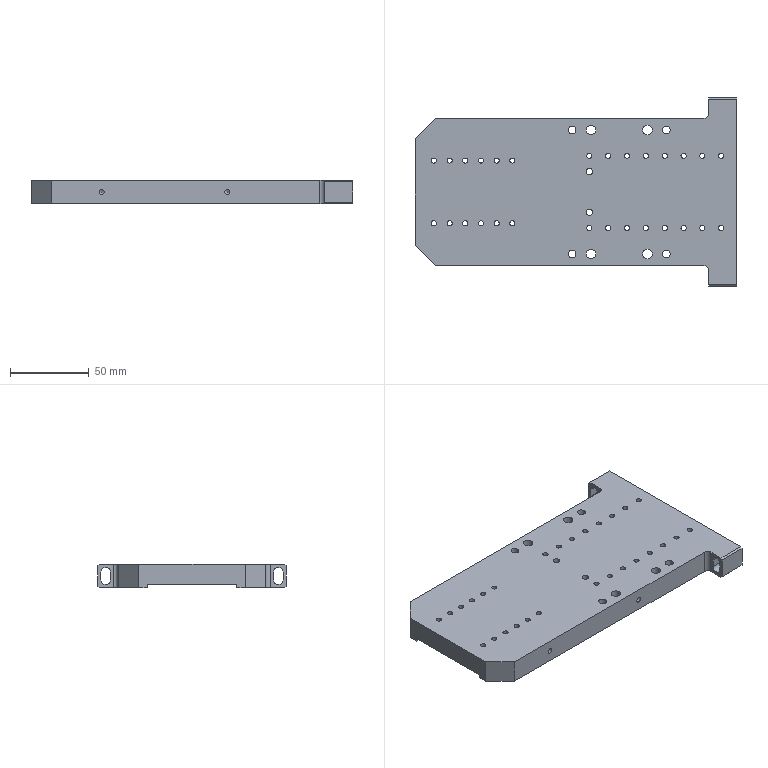CAM job | NX | 3-axis milling, drilling | part box 205 x 120 x 15 mm | stock box 210 x 120 x 20 mm
Tools:
number,name,description,diameter,corner_radius,flute_length,length,flutes
9,D10,平底铣刀-粗,10.0,0.0,35.0,75.0,2
7,D6-J,平底铣刀-精,6.0,0.0,25.0,75.0,2
10,D10-J,平底铣刀-精,10.0,0.0,35.0,75.0,2
1,D80R0.8FLYCUTTER,圆鼻刀-粗,80.0,0.8,50.0,75.0,2
1,D80R0.8FLYCUTTER-J,圆鼻刀-精,80.0,0.8,50.0,75.0,2
2,D6CHAMFERTOOL,倒角刀,6.0,0.0,3.0,25.0,2
21,M4X0.7,丝锥,3.3,0.0,35.0,50.0,2
23,M6X1.0,丝锥,5.0,0.0,35.0,50.0,2
19,D4REAMER,Drilling Tool,4.0,0.0,75.0,100.0,6
20,D6REAMER,Drilling Tool,6.0,0.0,75.0,100.0,6
15,ZT5,钻头,5.0,0.0,35.0,50.0,2
13,DRILL3.3,Twist Drill 3.3 mm,3.3,0.0,35.0,35.008,2
17,ZT3.9,Drilling Tool,3.9,0.0,35.0,50.0,2
18,ZT5.9,Drilling Tool,5.9,0.0,35.0,50.0,2
Operations:
program,operation,operation_type,tool,method,geometry_group,spindle_rpm,surface_speed,feed_per_tooth,feed_cut,feed_plunge,cut_length_mm,path_length_mm,cut_time_min,machine_time_min
A,TOPFACE,FaceMilling,D80R0.8FLYCUTTER,SIDEFINISH-DEPTHK-STEPG,W-A,4000.0,1005.28,0.125,1000.0,100.0,650.667,686.667,0.6507,0.6543
A,DYNROUGHD10_COPY,CavityMilling,D10,DYNROUGH-DEPTHK-STEPK,W-A,8000.0,251.32,0.25,4000.0,100.0,9574.982,10367.502,2.394,2.473
A,FLOORWALLROUGH_1,VolumeBased25DMillingOperation,D10,METHOD,W-A,6000.0,113.0,0.2083,3500.0,100.0,6895.6,7025.263,1.97,1.983
A,SPOT-DEPTH0.8,Operation,D6CHAMFERTOOL,NONE,W-A,8000.0,150.796,0.0312,500.0,90.0,68.4,763.92,0.1368,0.2064
A,THRUHOLE-M4TAPDRILL,Operation,DRILL3.3,NONE,W-A,3000.0,31.102,0.05,300.0,90.0,559.76,1594.726,1.866,1.969
A,THRUHOLE-FINEHOLE4.0PREDRILL,Operation,ZT3.9,NONE,W-A,3000.0,36.757,0.0417,250.0,90.0,36.252,143.523,0.145,0.1557
A,THRUHOLE-M6TAPDRILL,Operation,ZT5,NONE,W-A,2800.0,43.982,0.0625,350.0,90.0,94.009,430.04,0.2686,0.3022
A,THRUHOLE-FINEHOLE6.0PREDRILL,Operation,ZT5.9,NONE,W-A,2500.0,46.339,0.05,250.0,90.0,82.813,359.66,0.3313,0.3589
A,FLOORFINISH_1,VolumeBased25DMillingOperation,D10-J,METHOD,W-A,6000.0,113.0,0.2083,1200.0,100.0,1773.999,1816.999,1.478,1.483
A,PROFILESIDE,ZLevelMilling,D6-J,METHOD,W-A,9000.0,84.823,0.1389,2500.0,80.0,858.402,1070.933,0.3437,0.3649
A,SELBODYONLY,SurfaceContour,D6CHAMFERTOOL,METHOD,W-A,8000.0,150.796,0.1875,3000.0,100.0,1041.766,1717.404,0.3473,0.4148
A,DRILLCHAMFER_1,Operation,D6CHAMFERTOOL,METHOD,W-A,8000.0,150.796,0.0312,500.0,0.0,145.6,829.167,0.2912,0.3596
A,DRILLCHAMFER_2,Operation,D6CHAMFERTOOL,METHOD,W-A,8000.0,150.796,0.0312,500.0,0.0,10.6,94.373,0.0212,0.0296
A,MILLCHAMFER_1,PlanarMilling,D6CHAMFERTOOL,METHOD,W-A,8000.0,150.796,0.0312,500.0,100.0,79.753,441.58,0.1595,0.1957
A,MILLCHAMFER_2,PlanarMilling,D6CHAMFERTOOL,METHOD,W-A,8000.0,150.796,0.0312,500.0,100.0,83.855,396.707,0.1677,0.199
A,FLOORWALLCHAMFER_COPY,VolumeBased25DMillingOperation,D6CHAMFERTOOL,WALLCHAMFER-DEPTH0-STEPG,W-A,6500.0,122.519,0.1154,1500.0,100.0,53.601,255.817,0.0357,0.056
A,REAM,Operation,D4REAMER,METHOD,W-A,500.0,6.283,0.0167,50.0,0.0,30.0,131.019,0.6,0.6101
A,REAM_2,Operation,D6REAMER,METHOD,W-A,500.0,9.425,0.0167,50.0,0.0,68.0,330.034,1.36,1.386
A,THRUHOLE-TAPM4,Operation,M4X0.7,METHOD,W-A,600.0,6.22,0.0006,0.7,90.0,476.0,1427.206,680.0,680.095
A,THRUHOLE-TAPM6,Operation,M6X1.0,METHOD,W-A,500.0,7.854,0.001,1.0,90.0,78.0,398.023,78.0,78.032
A,FLOORSIDEFINISH_3,VolumeBased25DMillingOperation,D10-J,METHOD,W-A,6000.0,113.0,0.2083,1200.0,100.0,436.683,567.523,0.3639,0.377
A,PROFILESEMI_2,VolumeBased25DMillingOperation,D6-J,METHOD,W-A,6000.0,188.496,0.0833,1000.0,100.0,655.96,725.56,0.656,0.6629
B,FLOORWALLFACEROUGH_COPY,VolumeBased25DMillingOperation,D80R0.8FLYCUTTER,LAYERROUGH-DEPTHK-STEPG,W-B,5000.0,1256.637,0.3,3000.0,100.0,5907.187,6517.757,1.969,2.03
B,FLOORWALLFACEFINISH_COPY,VolumeBased25DMillingOperation,D80R0.8FLYCUTTER-J,SIDEFINISH-DEPTHK-STEPG,W-B,5000.0,1256.637,0.1,1000.0,100.0,655.766,751.766,0.6558,0.6654
B,DRILLCHAMFER_3,Operation,D6CHAMFERTOOL,METHOD,W-B,8000.0,150.796,0.0625,1000.0,0.0,145.6,825.167,0.1456,0.2136
B,DRILLCHAMFER_4,Operation,D6CHAMFERTOOL,METHOD,W-B,8000.0,150.796,0.0625,1000.0,0.0,10.6,90.373,0.0106,0.0186
B,MILLCHAMFER_3,PlanarMilling,D6CHAMFERTOOL,METHOD,W-B,8000.0,150.796,0.0375,600.0,100.0,75.821,680.332,0.1264,0.1868
B,MILLCHAMFER_4,PlanarMilling,D6CHAMFERTOOL,METHOD,W-B,8000.0,150.796,0.0375,600.0,100.0,75.821,635.844,0.1264,0.1824
B,C0.3CLOSEDCONTOURCHAMFER6X45L_COPY,PlanarMilling,D6CHAMFERTOOL,WALLCHAMFER-DEPTH0-STEPG,W-B,7000.0,131.0,0.1071,1500.0,100.0,649.259,745.259,0.4328,0.4424
B,FLOORWALLCHAMFER_COPY_1,VolumeBased25DMillingOperation,D6CHAMFERTOOL,WALLCHAMFER-DEPTH0-STEPG,W-B,6500.0,122.519,0.1154,1500.0,100.0,53.601,375.817,0.0357,0.068